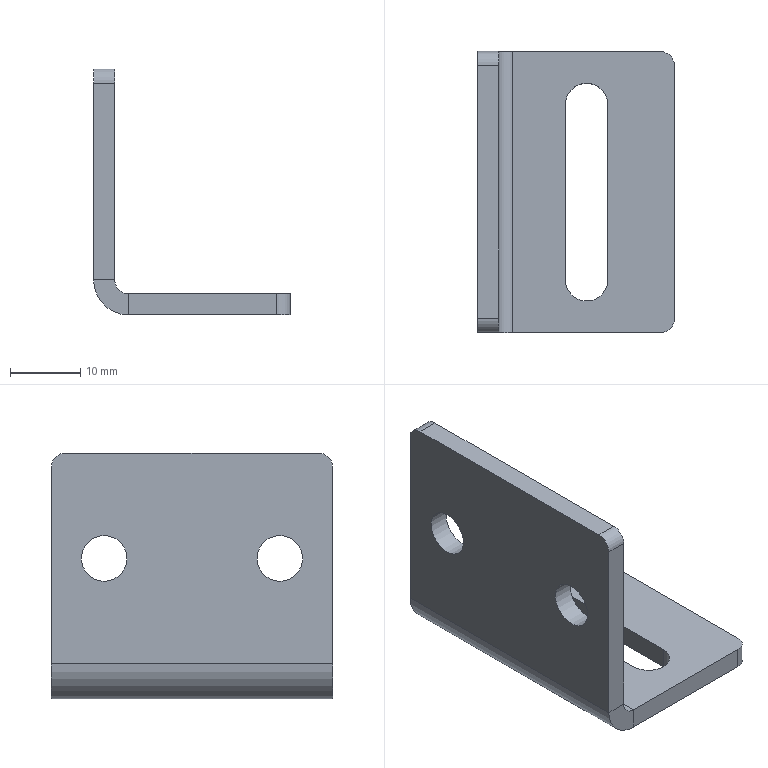Part | NX | 1 solid | 24 faces | box 28 x 40 x 35 mm | volume 6276 mm3 | plane 14 | cylinder 10 | commonest cylinder face diameters 4 x5 6 x2 6.5 x2 10 x1
STEP:
#1=CARTESIAN_POINT('',(0.,20.,2.));
#2=VERTEX_POINT('',#1);
#3=CARTESIAN_POINT('',(-3.,20.,2.));
#4=VERTEX_POINT('',#3);
#5=CARTESIAN_POINT('',(0.,20.,2.));
#6=DIRECTION('',(-1.,0.,0.));
#7=VECTOR('',#6,1000.);
#8=LINE('',#5,#7);
#9=EDGE_CURVE('',#2,#4,#8,.T.);
#10=ORIENTED_EDGE('',*,*,#9,.F.);
#11=CARTESIAN_POINT('',(2.,20.,0.));
#12=VERTEX_POINT('',#11);
#13=CARTESIAN_POINT('',(2.,20.,2.));
#14=DIRECTION('',(0.,-1.,0.));
#15=DIRECTION('',(0.,0.,-1.));
#16=AXIS2_PLACEMENT_3D('',#13,#14,#15);
#17=CIRCLE('',#16,2.);
#18=EDGE_CURVE('',#12,#2,#17,.F.);
#19=ORIENTED_EDGE('',*,*,#18,.F.);
#20=CARTESIAN_POINT('',(2.,20.,-3.));
#21=VERTEX_POINT('',#20);
#22=CARTESIAN_POINT('',(2.,20.,-3.));
#23=DIRECTION('',(0.,0.,1.));
#24=VECTOR('',#23,1000.);
#25=LINE('',#22,#24);
#26=EDGE_CURVE('',#21,#12,#25,.T.);
#27=ORIENTED_EDGE('',*,*,#26,.F.);
#28=CARTESIAN_POINT('',(2.,20.,2.));
#29=DIRECTION('',(0.,1.,0.));
#30=DIRECTION('',(1.,0.,0.));
#31=AXIS2_PLACEMENT_3D('',#28,#29,#30);
#32=CIRCLE('',#31,5.);
#33=EDGE_CURVE('',#21,#4,#32,.T.);
#34=ORIENTED_EDGE('',*,*,#33,.T.);
#35=EDGE_LOOP('',(#10,#19,#27,#34));
#36=FACE_BOUND('',#35,.T.);
#37=CARTESIAN_POINT('',(0.,20.,2.));
#38=DIRECTION('',(0.,1.,0.));
#39=DIRECTION('',(0.,0.,1.));
#40=AXIS2_PLACEMENT_3D('',#37,#38,#39);
#41=PLANE('',#40);
#42=ADVANCED_FACE('',(#36),#41,.T.);
#43=CARTESIAN_POINT('',(-3.,20.,30.));
#44=VERTEX_POINT('',#43);
#45=CARTESIAN_POINT('',(-3.,20.,0.));
#46=DIRECTION('',(0.,0.,1.));
#47=VECTOR('',#46,1000.);
#48=LINE('',#45,#47);
#49=EDGE_CURVE('',#4,#44,#48,.T.);
#50=ORIENTED_EDGE('',*,*,#49,.T.);
#51=CARTESIAN_POINT('',(0.,20.,30.));
#52=VERTEX_POINT('',#51);
#53=CARTESIAN_POINT('',(2.,20.,30.));
#54=DIRECTION('',(-1.,0.,0.));
#55=VECTOR('',#54,1000.);
#56=LINE('',#53,#55);
#57=EDGE_CURVE('',#44,#52,#56,.F.);
#58=ORIENTED_EDGE('',*,*,#57,.T.);
#59=CARTESIAN_POINT('',(0.,20.,0.));
#60=DIRECTION('',(0.,0.,1.));
#61=VECTOR('',#60,1000.);
#62=LINE('',#59,#61);
#63=EDGE_CURVE('',#2,#52,#62,.T.);
#64=ORIENTED_EDGE('',*,*,#63,.F.);
#65=ORIENTED_EDGE('',*,*,#9,.T.);
#66=EDGE_LOOP('',(#50,#58,#64,#65));
#67=FACE_BOUND('',#66,.T.);
#68=CARTESIAN_POINT('',(2.,20.,-3.));
#69=DIRECTION('',(0.,1.,0.));
#70=DIRECTION('',(0.,0.,1.));
#71=AXIS2_PLACEMENT_3D('',#68,#69,#70);
#72=PLANE('',#71);
#73=ADVANCED_FACE('',(#67),#72,.T.);
#74=CARTESIAN_POINT('',(2.,-20.,0.));
#75=VERTEX_POINT('',#74);
#76=CARTESIAN_POINT('',(2.,-20.,-3.));
#77=VERTEX_POINT('',#76);
#78=CARTESIAN_POINT('',(2.,-20.,0.));
#79=DIRECTION('',(0.,0.,-1.));
#80=VECTOR('',#79,1000.);
#81=LINE('',#78,#80);
#82=EDGE_CURVE('',#75,#77,#81,.T.);
#83=ORIENTED_EDGE('',*,*,#82,.F.);
#84=CARTESIAN_POINT('',(0.,-20.,2.));
#85=VERTEX_POINT('',#84);
#86=CARTESIAN_POINT('',(2.,-20.,2.));
#87=DIRECTION('',(0.,-1.,0.));
#88=DIRECTION('',(0.,0.,-1.));
#89=AXIS2_PLACEMENT_3D('',#86,#87,#88);
#90=CIRCLE('',#89,2.);
#91=EDGE_CURVE('',#75,#85,#90,.F.);
#92=ORIENTED_EDGE('',*,*,#91,.T.);
#93=CARTESIAN_POINT('',(-3.,-20.,2.));
#94=VERTEX_POINT('',#93);
#95=CARTESIAN_POINT('',(-3.,-20.,2.));
#96=DIRECTION('',(1.,0.,0.));
#97=VECTOR('',#96,1000.);
#98=LINE('',#95,#97);
#99=EDGE_CURVE('',#94,#85,#98,.T.);
#100=ORIENTED_EDGE('',*,*,#99,.F.);
#101=CARTESIAN_POINT('',(2.,-20.,2.));
#102=DIRECTION('',(0.,1.,0.));
#103=DIRECTION('',(1.,0.,0.));
#104=AXIS2_PLACEMENT_3D('',#101,#102,#103);
#105=CIRCLE('',#104,5.);
#106=EDGE_CURVE('',#77,#94,#105,.T.);
#107=ORIENTED_EDGE('',*,*,#106,.F.);
#108=EDGE_LOOP('',(#83,#92,#100,#107));
#109=FACE_BOUND('',#108,.T.);
#110=CARTESIAN_POINT('',(2.,-20.,0.));
#111=DIRECTION('',(0.,-1.,0.));
#112=DIRECTION('',(0.,0.,-1.));
#113=AXIS2_PLACEMENT_3D('',#110,#111,#112);
#114=PLANE('',#113);
#115=ADVANCED_FACE('',(#109),#114,.T.);
#116=CARTESIAN_POINT('',(23.,-20.,-3.));
#117=VERTEX_POINT('',#116);
#118=CARTESIAN_POINT('',(25.,-20.,-3.));
#119=DIRECTION('',(-1.,0.,0.));
#120=VECTOR('',#119,1000.);
#121=LINE('',#118,#120);
#122=EDGE_CURVE('',#117,#77,#121,.T.);
#123=ORIENTED_EDGE('',*,*,#122,.F.);
#124=CARTESIAN_POINT('',(23.,-20.,0.));
#125=VERTEX_POINT('',#124);
#126=CARTESIAN_POINT('',(23.,-20.,2.));
#127=DIRECTION('',(0.,0.,1.));
#128=VECTOR('',#127,1000.);
#129=LINE('',#126,#128);
#130=EDGE_CURVE('',#117,#125,#129,.T.);
#131=ORIENTED_EDGE('',*,*,#130,.T.);
#132=CARTESIAN_POINT('',(25.,-20.,0.));
#133=DIRECTION('',(-1.,0.,0.));
#134=VECTOR('',#133,1000.);
#135=LINE('',#132,#134);
#136=EDGE_CURVE('',#125,#75,#135,.T.);
#137=ORIENTED_EDGE('',*,*,#136,.T.);
#138=ORIENTED_EDGE('',*,*,#82,.T.);
#139=EDGE_LOOP('',(#123,#131,#137,#138));
#140=FACE_BOUND('',#139,.T.);
#141=CARTESIAN_POINT('',(-3.,-20.,2.));
#142=DIRECTION('',(0.,-1.,0.));
#143=DIRECTION('',(0.,0.,-1.));
#144=AXIS2_PLACEMENT_3D('',#141,#142,#143);
#145=PLANE('',#144);
#146=ADVANCED_FACE('',(#140),#145,.T.);
#147=CARTESIAN_POINT('',(-3.,-12.5,20.25));
#148=VERTEX_POINT('',#147);
#149=CARTESIAN_POINT('',(-3.,-12.5,17.));
#150=DIRECTION('',(-1.,0.,0.));
#151=DIRECTION('',(0.,0.,1.));
#152=AXIS2_PLACEMENT_3D('',#149,#150,#151);
#153=CIRCLE('',#152,3.25);
#154=EDGE_CURVE('',#148,#148,#153,.T.);
#155=ORIENTED_EDGE('',*,*,#154,.F.);
#156=EDGE_LOOP('',(#155));
#157=FACE_BOUND('',#156,.T.);
#158=CARTESIAN_POINT('',(-3.,12.5,20.25));
#159=VERTEX_POINT('',#158);
#160=CARTESIAN_POINT('',(-3.,12.5,17.));
#161=DIRECTION('',(-1.,0.,0.));
#162=DIRECTION('',(0.,0.,1.));
#163=AXIS2_PLACEMENT_3D('',#160,#161,#162);
#164=CIRCLE('',#163,3.25);
#165=EDGE_CURVE('',#159,#159,#164,.T.);
#166=ORIENTED_EDGE('',*,*,#165,.F.);
#167=EDGE_LOOP('',(#166));
#168=FACE_BOUND('',#167,.T.);
#169=CARTESIAN_POINT('',(-3.,18.,32.));
#170=VERTEX_POINT('',#169);
#171=CARTESIAN_POINT('',(-3.,-18.,32.));
#172=VERTEX_POINT('',#171);
#173=CARTESIAN_POINT('',(-3.,20.,32.));
#174=DIRECTION('',(0.,-1.,0.));
#175=VECTOR('',#174,1000.);
#176=LINE('',#173,#175);
#177=EDGE_CURVE('',#170,#172,#176,.T.);
#178=ORIENTED_EDGE('',*,*,#177,.F.);
#179=CARTESIAN_POINT('',(-3.,18.,30.));
#180=DIRECTION('',(1.,0.,0.));
#181=DIRECTION('',(0.,0.,-1.));
#182=AXIS2_PLACEMENT_3D('',#179,#180,#181);
#183=CIRCLE('',#182,2.);
#184=EDGE_CURVE('',#170,#44,#183,.F.);
#185=ORIENTED_EDGE('',*,*,#184,.T.);
#186=ORIENTED_EDGE('',*,*,#49,.F.);
#187=CARTESIAN_POINT('',(-3.,20.,2.));
#188=DIRECTION('',(0.,-1.,0.));
#189=VECTOR('',#188,1000.);
#190=LINE('',#187,#189);
#191=EDGE_CURVE('',#4,#94,#190,.T.);
#192=ORIENTED_EDGE('',*,*,#191,.T.);
#193=CARTESIAN_POINT('',(-3.,-20.,30.));
#194=VERTEX_POINT('',#193);
#195=CARTESIAN_POINT('',(-3.,-20.,0.));
#196=DIRECTION('',(0.,0.,1.));
#197=VECTOR('',#196,1000.);
#198=LINE('',#195,#197);
#199=EDGE_CURVE('',#94,#194,#198,.T.);
#200=ORIENTED_EDGE('',*,*,#199,.T.);
#201=CARTESIAN_POINT('',(-3.,-18.,30.));
#202=DIRECTION('',(1.,0.,0.));
#203=DIRECTION('',(0.,0.,-1.));
#204=AXIS2_PLACEMENT_3D('',#201,#202,#203);
#205=CIRCLE('',#204,2.);
#206=EDGE_CURVE('',#194,#172,#205,.F.);
#207=ORIENTED_EDGE('',*,*,#206,.T.);
#208=EDGE_LOOP('',(#178,#185,#186,#192,#200,#207));
#209=FACE_BOUND('',#208,.T.);
#210=CARTESIAN_POINT('',(-3.,20.,0.));
#211=DIRECTION('',(1.,0.,0.));
#212=DIRECTION('',(0.,0.,-1.));
#213=AXIS2_PLACEMENT_3D('',#210,#211,#212);
#214=PLANE('',#213);
#215=ADVANCED_FACE('',(#157,#168,#209),#214,.F.);
#216=CARTESIAN_POINT('',(0.,18.,32.));
#217=VERTEX_POINT('',#216);
#218=CARTESIAN_POINT('',(0.,-18.,32.));
#219=VERTEX_POINT('',#218);
#220=CARTESIAN_POINT('',(0.,20.,32.));
#221=DIRECTION('',(0.,-1.,0.));
#222=VECTOR('',#221,1000.);
#223=LINE('',#220,#222);
#224=EDGE_CURVE('',#217,#219,#223,.T.);
#225=ORIENTED_EDGE('',*,*,#224,.F.);
#226=CARTESIAN_POINT('',(0.,18.,32.));
#227=DIRECTION('',(-1.,0.,0.));
#228=VECTOR('',#227,1000.);
#229=LINE('',#226,#228);
#230=EDGE_CURVE('',#217,#170,#229,.T.);
#231=ORIENTED_EDGE('',*,*,#230,.T.);
#232=ORIENTED_EDGE('',*,*,#177,.T.);
#233=CARTESIAN_POINT('',(0.,-18.,32.));
#234=DIRECTION('',(-1.,0.,0.));
#235=VECTOR('',#234,1000.);
#236=LINE('',#233,#235);
#237=EDGE_CURVE('',#172,#219,#236,.F.);
#238=ORIENTED_EDGE('',*,*,#237,.T.);
#239=EDGE_LOOP('',(#225,#231,#232,#238));
#240=FACE_BOUND('',#239,.T.);
#241=CARTESIAN_POINT('',(0.,20.,32.));
#242=DIRECTION('',(0.,0.,1.));
#243=DIRECTION('',(1.,0.,0.));
#244=AXIS2_PLACEMENT_3D('',#241,#242,#243);
#245=PLANE('',#244);
#246=ADVANCED_FACE('',(#240),#245,.T.);
#247=CARTESIAN_POINT('',(0.,-12.5,13.75));
#248=VERTEX_POINT('',#247);
#249=CARTESIAN_POINT('',(0.,-12.5,17.));
#250=DIRECTION('',(1.,0.,0.));
#251=DIRECTION('',(0.,0.,-1.));
#252=AXIS2_PLACEMENT_3D('',#249,#250,#251);
#253=CIRCLE('',#252,3.25);
#254=EDGE_CURVE('',#248,#248,#253,.T.);
#255=ORIENTED_EDGE('',*,*,#254,.F.);
#256=EDGE_LOOP('',(#255));
#257=FACE_BOUND('',#256,.T.);
#258=CARTESIAN_POINT('',(0.,12.5,13.75));
#259=VERTEX_POINT('',#258);
#260=CARTESIAN_POINT('',(0.,12.5,17.));
#261=DIRECTION('',(1.,0.,0.));
#262=DIRECTION('',(0.,0.,-1.));
#263=AXIS2_PLACEMENT_3D('',#260,#261,#262);
#264=CIRCLE('',#263,3.25);
#265=EDGE_CURVE('',#259,#259,#264,.T.);
#266=ORIENTED_EDGE('',*,*,#265,.F.);
#267=EDGE_LOOP('',(#266));
#268=FACE_BOUND('',#267,.T.);
#269=ORIENTED_EDGE('',*,*,#63,.T.);
#270=CARTESIAN_POINT('',(0.,18.,30.));
#271=DIRECTION('',(1.,0.,0.));
#272=DIRECTION('',(0.,0.,-1.));
#273=AXIS2_PLACEMENT_3D('',#270,#271,#272);
#274=CIRCLE('',#273,2.);
#275=EDGE_CURVE('',#52,#217,#274,.T.);
#276=ORIENTED_EDGE('',*,*,#275,.T.);
#277=ORIENTED_EDGE('',*,*,#224,.T.);
#278=CARTESIAN_POINT('',(0.,-20.,30.));
#279=VERTEX_POINT('',#278);
#280=CARTESIAN_POINT('',(0.,-18.,30.));
#281=DIRECTION('',(1.,0.,0.));
#282=DIRECTION('',(0.,0.,-1.));
#283=AXIS2_PLACEMENT_3D('',#280,#281,#282);
#284=CIRCLE('',#283,2.);
#285=EDGE_CURVE('',#219,#279,#284,.T.);
#286=ORIENTED_EDGE('',*,*,#285,.T.);
#287=CARTESIAN_POINT('',(0.,-20.,0.));
#288=DIRECTION('',(0.,0.,1.));
#289=VECTOR('',#288,1000.);
#290=LINE('',#287,#289);
#291=EDGE_CURVE('',#85,#279,#290,.T.);
#292=ORIENTED_EDGE('',*,*,#291,.F.);
#293=CARTESIAN_POINT('',(0.,20.,2.));
#294=DIRECTION('',(0.,-1.,0.));
#295=VECTOR('',#294,1000.);
#296=LINE('',#293,#295);
#297=EDGE_CURVE('',#2,#85,#296,.T.);
#298=ORIENTED_EDGE('',*,*,#297,.F.);
#299=EDGE_LOOP('',(#269,#276,#277,#286,#292,#298));
#300=FACE_BOUND('',#299,.T.);
#301=CARTESIAN_POINT('',(0.,20.,0.));
#302=DIRECTION('',(1.,0.,0.));
#303=DIRECTION('',(0.,0.,-1.));
#304=AXIS2_PLACEMENT_3D('',#301,#302,#303);
#305=PLANE('',#304);
#306=ADVANCED_FACE('',(#257,#268,#300),#305,.T.);
#307=ORIENTED_EDGE('',*,*,#91,.F.);
#308=CARTESIAN_POINT('',(2.,20.,0.));
#309=DIRECTION('',(0.,-1.,0.));
#310=VECTOR('',#309,1000.);
#311=LINE('',#308,#310);
#312=EDGE_CURVE('',#12,#75,#311,.T.);
#313=ORIENTED_EDGE('',*,*,#312,.F.);
#314=ORIENTED_EDGE('',*,*,#18,.T.);
#315=ORIENTED_EDGE('',*,*,#297,.T.);
#316=EDGE_LOOP('',(#307,#313,#314,#315));
#317=FACE_BOUND('',#316,.T.);
#318=CARTESIAN_POINT('',(2.,20.,2.));
#319=DIRECTION('',(0.,-1.,0.));
#320=DIRECTION('',(0.,0.,-1.));
#321=AXIS2_PLACEMENT_3D('',#318,#319,#320);
#322=CYLINDRICAL_SURFACE('',#321,2.);
#323=ADVANCED_FACE('',(#317),#322,.F.);
#324=CARTESIAN_POINT('',(15.5,12.5,0.));
#325=VERTEX_POINT('',#324);
#326=CARTESIAN_POINT('',(9.5,12.5,0.));
#327=VERTEX_POINT('',#326);
#328=CARTESIAN_POINT('',(12.5,12.5,0.));
#329=DIRECTION('',(0.,0.,1.));
#330=DIRECTION('',(1.,0.,0.));
#331=AXIS2_PLACEMENT_3D('',#328,#329,#330);
#332=CIRCLE('',#331,3.);
#333=EDGE_CURVE('',#325,#327,#332,.T.);
#334=ORIENTED_EDGE('',*,*,#333,.F.);
#335=CARTESIAN_POINT('',(15.5,-12.5,0.));
#336=VERTEX_POINT('',#335);
#337=CARTESIAN_POINT('',(15.5,20.,0.));
#338=DIRECTION('',(0.,1.,0.));
#339=VECTOR('',#338,1000.);
#340=LINE('',#337,#339);
#341=EDGE_CURVE('',#336,#325,#340,.T.);
#342=ORIENTED_EDGE('',*,*,#341,.F.);
#343=CARTESIAN_POINT('',(9.5,-12.5,0.));
#344=VERTEX_POINT('',#343);
#345=CARTESIAN_POINT('',(12.5,-12.5,0.));
#346=DIRECTION('',(0.,0.,1.));
#347=DIRECTION('',(1.,0.,0.));
#348=AXIS2_PLACEMENT_3D('',#345,#346,#347);
#349=CIRCLE('',#348,3.);
#350=EDGE_CURVE('',#344,#336,#349,.T.);
#351=ORIENTED_EDGE('',*,*,#350,.F.);
#352=CARTESIAN_POINT('',(9.5,20.,0.));
#353=DIRECTION('',(0.,-1.,0.));
#354=VECTOR('',#353,1000.);
#355=LINE('',#352,#354);
#356=EDGE_CURVE('',#327,#344,#355,.T.);
#357=ORIENTED_EDGE('',*,*,#356,.F.);
#358=EDGE_LOOP('',(#334,#342,#351,#357));
#359=FACE_BOUND('',#358,.T.);
#360=ORIENTED_EDGE('',*,*,#136,.F.);
#361=CARTESIAN_POINT('',(25.,-18.,0.));
#362=VERTEX_POINT('',#361);
#363=CARTESIAN_POINT('',(23.,-18.,0.));
#364=DIRECTION('',(0.,0.,1.));
#365=DIRECTION('',(1.,0.,0.));
#366=AXIS2_PLACEMENT_3D('',#363,#364,#365);
#367=CIRCLE('',#366,2.);
#368=EDGE_CURVE('',#125,#362,#367,.T.);
#369=ORIENTED_EDGE('',*,*,#368,.T.);
#370=CARTESIAN_POINT('',(25.,18.,0.));
#371=VERTEX_POINT('',#370);
#372=CARTESIAN_POINT('',(25.,20.,0.));
#373=DIRECTION('',(0.,-1.,0.));
#374=VECTOR('',#373,1000.);
#375=LINE('',#372,#374);
#376=EDGE_CURVE('',#371,#362,#375,.T.);
#377=ORIENTED_EDGE('',*,*,#376,.F.);
#378=CARTESIAN_POINT('',(23.,20.,0.));
#379=VERTEX_POINT('',#378);
#380=CARTESIAN_POINT('',(23.,18.,0.));
#381=DIRECTION('',(0.,0.,1.));
#382=DIRECTION('',(1.,0.,0.));
#383=AXIS2_PLACEMENT_3D('',#380,#381,#382);
#384=CIRCLE('',#383,2.);
#385=EDGE_CURVE('',#371,#379,#384,.T.);
#386=ORIENTED_EDGE('',*,*,#385,.T.);
#387=CARTESIAN_POINT('',(25.,20.,0.));
#388=DIRECTION('',(-1.,0.,0.));
#389=VECTOR('',#388,1000.);
#390=LINE('',#387,#389);
#391=EDGE_CURVE('',#379,#12,#390,.T.);
#392=ORIENTED_EDGE('',*,*,#391,.T.);
#393=ORIENTED_EDGE('',*,*,#312,.T.);
#394=EDGE_LOOP('',(#360,#369,#377,#386,#392,#393));
#395=FACE_BOUND('',#394,.T.);
#396=CARTESIAN_POINT('',(25.,20.,0.));
#397=DIRECTION('',(0.,0.,1.));
#398=DIRECTION('',(1.,0.,0.));
#399=AXIS2_PLACEMENT_3D('',#396,#397,#398);
#400=PLANE('',#399);
#401=ADVANCED_FACE('',(#359,#395),#400,.T.);
#402=ORIENTED_EDGE('',*,*,#376,.T.);
#403=CARTESIAN_POINT('',(25.,-18.,-3.));
#404=VERTEX_POINT('',#403);
#405=CARTESIAN_POINT('',(25.,-18.,-3.));
#406=DIRECTION('',(0.,0.,1.));
#407=VECTOR('',#406,1000.);
#408=LINE('',#405,#407);
#409=EDGE_CURVE('',#362,#404,#408,.F.);
#410=ORIENTED_EDGE('',*,*,#409,.T.);
#411=CARTESIAN_POINT('',(25.,18.,-3.));
#412=VERTEX_POINT('',#411);
#413=CARTESIAN_POINT('',(25.,20.,-3.));
#414=DIRECTION('',(0.,-1.,0.));
#415=VECTOR('',#414,1000.);
#416=LINE('',#413,#415);
#417=EDGE_CURVE('',#412,#404,#416,.T.);
#418=ORIENTED_EDGE('',*,*,#417,.F.);
#419=CARTESIAN_POINT('',(25.,18.,0.));
#420=DIRECTION('',(0.,0.,1.));
#421=VECTOR('',#420,1000.);
#422=LINE('',#419,#421);
#423=EDGE_CURVE('',#412,#371,#422,.T.);
#424=ORIENTED_EDGE('',*,*,#423,.T.);
#425=EDGE_LOOP('',(#402,#410,#418,#424));
#426=FACE_BOUND('',#425,.T.);
#427=CARTESIAN_POINT('',(25.,20.,-3.));
#428=DIRECTION('',(1.,0.,0.));
#429=DIRECTION('',(0.,0.,-1.));
#430=AXIS2_PLACEMENT_3D('',#427,#428,#429);
#431=PLANE('',#430);
#432=ADVANCED_FACE('',(#426),#431,.T.);
#433=CARTESIAN_POINT('',(15.5,12.5,-3.));
#434=VERTEX_POINT('',#433);
#435=CARTESIAN_POINT('',(15.5,-12.5,-3.));
#436=VERTEX_POINT('',#435);
#437=CARTESIAN_POINT('',(15.5,12.5,-3.));
#438=DIRECTION('',(0.,-1.,0.));
#439=VECTOR('',#438,1000.);
#440=LINE('',#437,#439);
#441=EDGE_CURVE('',#434,#436,#440,.T.);
#442=ORIENTED_EDGE('',*,*,#441,.F.);
#443=CARTESIAN_POINT('',(9.5,12.5,-3.));
#444=VERTEX_POINT('',#443);
#445=CARTESIAN_POINT('',(12.5,12.5,-3.));
#446=DIRECTION('',(0.,0.,-1.));
#447=DIRECTION('',(-1.,0.,0.));
#448=AXIS2_PLACEMENT_3D('',#445,#446,#447);
#449=CIRCLE('',#448,3.);
#450=EDGE_CURVE('',#444,#434,#449,.T.);
#451=ORIENTED_EDGE('',*,*,#450,.F.);
#452=CARTESIAN_POINT('',(9.5,-12.5,-3.));
#453=VERTEX_POINT('',#452);
#454=CARTESIAN_POINT('',(9.5,12.5,-3.));
#455=DIRECTION('',(0.,1.,0.));
#456=VECTOR('',#455,1000.);
#457=LINE('',#454,#456);
#458=EDGE_CURVE('',#453,#444,#457,.T.);
#459=ORIENTED_EDGE('',*,*,#458,.F.);
#460=CARTESIAN_POINT('',(12.5,-12.5,-3.));
#461=DIRECTION('',(0.,0.,-1.));
#462=DIRECTION('',(-1.,0.,0.));
#463=AXIS2_PLACEMENT_3D('',#460,#461,#462);
#464=CIRCLE('',#463,3.);
#465=EDGE_CURVE('',#436,#453,#464,.T.);
#466=ORIENTED_EDGE('',*,*,#465,.F.);
#467=EDGE_LOOP('',(#442,#451,#459,#466));
#468=FACE_BOUND('',#467,.T.);
#469=ORIENTED_EDGE('',*,*,#417,.T.);
#470=CARTESIAN_POINT('',(23.,-18.,-3.));
#471=DIRECTION('',(0.,0.,1.));
#472=DIRECTION('',(1.,0.,0.));
#473=AXIS2_PLACEMENT_3D('',#470,#471,#472);
#474=CIRCLE('',#473,2.);
#475=EDGE_CURVE('',#404,#117,#474,.F.);
#476=ORIENTED_EDGE('',*,*,#475,.T.);
#477=ORIENTED_EDGE('',*,*,#122,.T.);
#478=CARTESIAN_POINT('',(2.,20.,-3.));
#479=DIRECTION('',(0.,-1.,0.));
#480=VECTOR('',#479,1000.);
#481=LINE('',#478,#480);
#482=EDGE_CURVE('',#21,#77,#481,.T.);
#483=ORIENTED_EDGE('',*,*,#482,.F.);
#484=CARTESIAN_POINT('',(23.,20.,-3.));
#485=VERTEX_POINT('',#484);
#486=CARTESIAN_POINT('',(25.,20.,-3.));
#487=DIRECTION('',(-1.,0.,0.));
#488=VECTOR('',#487,1000.);
#489=LINE('',#486,#488);
#490=EDGE_CURVE('',#485,#21,#489,.T.);
#491=ORIENTED_EDGE('',*,*,#490,.F.);
#492=CARTESIAN_POINT('',(23.,18.,-3.));
#493=DIRECTION('',(0.,0.,1.));
#494=DIRECTION('',(1.,0.,0.));
#495=AXIS2_PLACEMENT_3D('',#492,#493,#494);
#496=CIRCLE('',#495,2.);
#497=EDGE_CURVE('',#485,#412,#496,.F.);
#498=ORIENTED_EDGE('',*,*,#497,.T.);
#499=EDGE_LOOP('',(#469,#476,#477,#483,#491,#498));
#500=FACE_BOUND('',#499,.T.);
#501=CARTESIAN_POINT('',(25.,20.,-3.));
#502=DIRECTION('',(0.,0.,1.));
#503=DIRECTION('',(1.,0.,0.));
#504=AXIS2_PLACEMENT_3D('',#501,#502,#503);
#505=PLANE('',#504);
#506=ADVANCED_FACE('',(#468,#500),#505,.F.);
#507=ORIENTED_EDGE('',*,*,#106,.T.);
#508=ORIENTED_EDGE('',*,*,#191,.F.);
#509=ORIENTED_EDGE('',*,*,#33,.F.);
#510=ORIENTED_EDGE('',*,*,#482,.T.);
#511=EDGE_LOOP('',(#507,#508,#509,#510));
#512=FACE_BOUND('',#511,.T.);
#513=CARTESIAN_POINT('',(2.,20.,2.));
#514=DIRECTION('',(0.,-1.,0.));
#515=DIRECTION('',(0.,0.,-1.));
#516=AXIS2_PLACEMENT_3D('',#513,#514,#515);
#517=CYLINDRICAL_SURFACE('',#516,5.);
#518=ADVANCED_FACE('',(#512),#517,.T.);
#519=ORIENTED_EDGE('',*,*,#391,.F.);
#520=CARTESIAN_POINT('',(23.,20.,-3.));
#521=DIRECTION('',(0.,0.,1.));
#522=VECTOR('',#521,1000.);
#523=LINE('',#520,#522);
#524=EDGE_CURVE('',#379,#485,#523,.F.);
#525=ORIENTED_EDGE('',*,*,#524,.T.);
#526=ORIENTED_EDGE('',*,*,#490,.T.);
#527=ORIENTED_EDGE('',*,*,#26,.T.);
#528=EDGE_LOOP('',(#519,#525,#526,#527));
#529=FACE_BOUND('',#528,.T.);
#530=CARTESIAN_POINT('',(2.,20.,2.));
#531=DIRECTION('',(0.,-1.,0.));
#532=DIRECTION('',(-1.,0.,0.));
#533=AXIS2_PLACEMENT_3D('',#530,#531,#532);
#534=PLANE('',#533);
#535=ADVANCED_FACE('',(#529),#534,.F.);
#536=ORIENTED_EDGE('',*,*,#291,.T.);
#537=CARTESIAN_POINT('',(2.,-20.,30.));
#538=DIRECTION('',(-1.,0.,0.));
#539=VECTOR('',#538,1000.);
#540=LINE('',#537,#539);
#541=EDGE_CURVE('',#279,#194,#540,.T.);
#542=ORIENTED_EDGE('',*,*,#541,.T.);
#543=ORIENTED_EDGE('',*,*,#199,.F.);
#544=ORIENTED_EDGE('',*,*,#99,.T.);
#545=EDGE_LOOP('',(#536,#542,#543,#544));
#546=FACE_BOUND('',#545,.T.);
#547=CARTESIAN_POINT('',(2.,-20.,2.));
#548=DIRECTION('',(0.,-1.,0.));
#549=DIRECTION('',(-1.,0.,0.));
#550=AXIS2_PLACEMENT_3D('',#547,#548,#549);
#551=PLANE('',#550);
#552=ADVANCED_FACE('',(#546),#551,.T.);
#553=ORIENTED_EDGE('',*,*,#265,.T.);
#554=EDGE_LOOP('',(#553));
#555=FACE_BOUND('',#554,.T.);
#556=ORIENTED_EDGE('',*,*,#165,.T.);
#557=EDGE_LOOP('',(#556));
#558=FACE_BOUND('',#557,.T.);
#559=CARTESIAN_POINT('',(-3.,12.5,17.));
#560=DIRECTION('',(-1.,0.,0.));
#561=DIRECTION('',(0.,0.,1.));
#562=AXIS2_PLACEMENT_3D('',#559,#560,#561);
#563=CYLINDRICAL_SURFACE('',#562,3.25);
#564=ADVANCED_FACE('',(#555,#558),#563,.F.);
#565=ORIENTED_EDGE('',*,*,#254,.T.);
#566=EDGE_LOOP('',(#565));
#567=FACE_BOUND('',#566,.T.);
#568=ORIENTED_EDGE('',*,*,#154,.T.);
#569=EDGE_LOOP('',(#568));
#570=FACE_BOUND('',#569,.T.);
#571=CARTESIAN_POINT('',(-3.,-12.5,17.));
#572=DIRECTION('',(-1.,0.,0.));
#573=DIRECTION('',(0.,0.,1.));
#574=AXIS2_PLACEMENT_3D('',#571,#572,#573);
#575=CYLINDRICAL_SURFACE('',#574,3.25);
#576=ADVANCED_FACE('',(#567,#570),#575,.F.);
#577=ORIENTED_EDGE('',*,*,#475,.F.);
#578=ORIENTED_EDGE('',*,*,#409,.F.);
#579=ORIENTED_EDGE('',*,*,#368,.F.);
#580=ORIENTED_EDGE('',*,*,#130,.F.);
#581=EDGE_LOOP('',(#577,#578,#579,#580));
#582=FACE_BOUND('',#581,.T.);
#583=CARTESIAN_POINT('',(23.,-18.,2.));
#584=DIRECTION('',(0.,0.,1.));
#585=DIRECTION('',(1.,0.,0.));
#586=AXIS2_PLACEMENT_3D('',#583,#584,#585);
#587=CYLINDRICAL_SURFACE('',#586,2.);
#588=ADVANCED_FACE('',(#582),#587,.T.);
#589=ORIENTED_EDGE('',*,*,#497,.F.);
#590=ORIENTED_EDGE('',*,*,#524,.F.);
#591=ORIENTED_EDGE('',*,*,#385,.F.);
#592=ORIENTED_EDGE('',*,*,#423,.F.);
#593=EDGE_LOOP('',(#589,#590,#591,#592));
#594=FACE_BOUND('',#593,.T.);
#595=CARTESIAN_POINT('',(23.,18.,-3.));
#596=DIRECTION('',(0.,0.,-1.));
#597=DIRECTION('',(-1.,0.,0.));
#598=AXIS2_PLACEMENT_3D('',#595,#596,#597);
#599=CYLINDRICAL_SURFACE('',#598,2.);
#600=ADVANCED_FACE('',(#594),#599,.T.);
#601=ORIENTED_EDGE('',*,*,#275,.F.);
#602=ORIENTED_EDGE('',*,*,#57,.F.);
#603=ORIENTED_EDGE('',*,*,#184,.F.);
#604=ORIENTED_EDGE('',*,*,#230,.F.);
#605=EDGE_LOOP('',(#601,#602,#603,#604));
#606=FACE_BOUND('',#605,.T.);
#607=CARTESIAN_POINT('',(0.,18.,30.));
#608=DIRECTION('',(-1.,0.,0.));
#609=DIRECTION('',(0.,0.,1.));
#610=AXIS2_PLACEMENT_3D('',#607,#608,#609);
#611=CYLINDRICAL_SURFACE('',#610,2.);
#612=ADVANCED_FACE('',(#606),#611,.T.);
#613=ORIENTED_EDGE('',*,*,#285,.F.);
#614=ORIENTED_EDGE('',*,*,#237,.F.);
#615=ORIENTED_EDGE('',*,*,#206,.F.);
#616=ORIENTED_EDGE('',*,*,#541,.F.);
#617=EDGE_LOOP('',(#613,#614,#615,#616));
#618=FACE_BOUND('',#617,.T.);
#619=CARTESIAN_POINT('',(2.,-18.,30.));
#620=DIRECTION('',(-1.,0.,0.));
#621=DIRECTION('',(0.,0.,1.));
#622=AXIS2_PLACEMENT_3D('',#619,#620,#621);
#623=CYLINDRICAL_SURFACE('',#622,2.);
#624=ADVANCED_FACE('',(#618),#623,.T.);
#625=ORIENTED_EDGE('',*,*,#333,.T.);
#626=CARTESIAN_POINT('',(9.5,12.5,32.));
#627=DIRECTION('',(0.,0.,-1.));
#628=VECTOR('',#627,1000.);
#629=LINE('',#626,#628);
#630=EDGE_CURVE('',#327,#444,#629,.T.);
#631=ORIENTED_EDGE('',*,*,#630,.T.);
#632=ORIENTED_EDGE('',*,*,#450,.T.);
#633=CARTESIAN_POINT('',(15.5,12.5,32.));
#634=DIRECTION('',(0.,0.,-1.));
#635=VECTOR('',#634,1000.);
#636=LINE('',#633,#635);
#637=EDGE_CURVE('',#325,#434,#636,.T.);
#638=ORIENTED_EDGE('',*,*,#637,.F.);
#639=EDGE_LOOP('',(#625,#631,#632,#638));
#640=FACE_BOUND('',#639,.T.);
#641=CARTESIAN_POINT('',(12.5,12.5,32.));
#642=DIRECTION('',(0.,0.,-1.));
#643=DIRECTION('',(-1.,0.,0.));
#644=AXIS2_PLACEMENT_3D('',#641,#642,#643);
#645=CYLINDRICAL_SURFACE('',#644,3.);
#646=ADVANCED_FACE('',(#640),#645,.F.);
#647=ORIENTED_EDGE('',*,*,#356,.T.);
#648=CARTESIAN_POINT('',(9.5,-12.5,32.));
#649=DIRECTION('',(0.,0.,-1.));
#650=VECTOR('',#649,1000.);
#651=LINE('',#648,#650);
#652=EDGE_CURVE('',#344,#453,#651,.T.);
#653=ORIENTED_EDGE('',*,*,#652,.T.);
#654=ORIENTED_EDGE('',*,*,#458,.T.);
#655=ORIENTED_EDGE('',*,*,#630,.F.);
#656=EDGE_LOOP('',(#647,#653,#654,#655));
#657=FACE_BOUND('',#656,.T.);
#658=CARTESIAN_POINT('',(9.5,12.5,32.));
#659=DIRECTION('',(-1.,0.,0.));
#660=DIRECTION('',(0.,0.,1.));
#661=AXIS2_PLACEMENT_3D('',#658,#659,#660);
#662=PLANE('',#661);
#663=ADVANCED_FACE('',(#657),#662,.F.);
#664=ORIENTED_EDGE('',*,*,#350,.T.);
#665=CARTESIAN_POINT('',(15.5,-12.5,32.));
#666=DIRECTION('',(0.,0.,-1.));
#667=VECTOR('',#666,1000.);
#668=LINE('',#665,#667);
#669=EDGE_CURVE('',#336,#436,#668,.T.);
#670=ORIENTED_EDGE('',*,*,#669,.T.);
#671=ORIENTED_EDGE('',*,*,#465,.T.);
#672=ORIENTED_EDGE('',*,*,#652,.F.);
#673=EDGE_LOOP('',(#664,#670,#671,#672));
#674=FACE_BOUND('',#673,.T.);
#675=CARTESIAN_POINT('',(12.5,-12.5,32.));
#676=DIRECTION('',(0.,0.,-1.));
#677=DIRECTION('',(-1.,0.,0.));
#678=AXIS2_PLACEMENT_3D('',#675,#676,#677);
#679=CYLINDRICAL_SURFACE('',#678,3.);
#680=ADVANCED_FACE('',(#674),#679,.F.);
#681=ORIENTED_EDGE('',*,*,#341,.T.);
#682=ORIENTED_EDGE('',*,*,#637,.T.);
#683=ORIENTED_EDGE('',*,*,#441,.T.);
#684=ORIENTED_EDGE('',*,*,#669,.F.);
#685=EDGE_LOOP('',(#681,#682,#683,#684));
#686=FACE_BOUND('',#685,.T.);
#687=CARTESIAN_POINT('',(15.5,12.5,32.));
#688=DIRECTION('',(1.,0.,0.));
#689=DIRECTION('',(0.,1.,0.));
#690=AXIS2_PLACEMENT_3D('',#687,#688,#689);
#691=PLANE('',#690);
#692=ADVANCED_FACE('',(#686),#691,.F.);
#693=CLOSED_SHELL('',(#42,#73,#115,#146,#215,#246,#306,#323,#401,#432,#506,#518,#535,#552,#564,#576,#588,#600,#612,#624,#646,#663,#680,#692));
#694=MANIFOLD_SOLID_BREP('',#693);
#695=(LENGTH_UNIT()NAMED_UNIT(*)SI_UNIT(.MILLI.,.METRE.));
#696=UNCERTAINTY_MEASURE_WITH_UNIT(LENGTH_MEASURE(0.00001),#695,'','');
#697=(NAMED_UNIT(*)PLANE_ANGLE_UNIT()SI_UNIT($,.RADIAN.));
#698=(NAMED_UNIT(*)SI_UNIT($,.STERADIAN.)SOLID_ANGLE_UNIT());
#699=(GEOMETRIC_REPRESENTATION_CONTEXT(3)GLOBAL_UNCERTAINTY_ASSIGNED_CONTEXT((#696))GLOBAL_UNIT_ASSIGNED_CONTEXT((#695,#697,#698))REPRESENTATION_CONTEXT('',''));
#700=ADVANCED_BREP_SHAPE_REPRESENTATION('',(#694),#699);